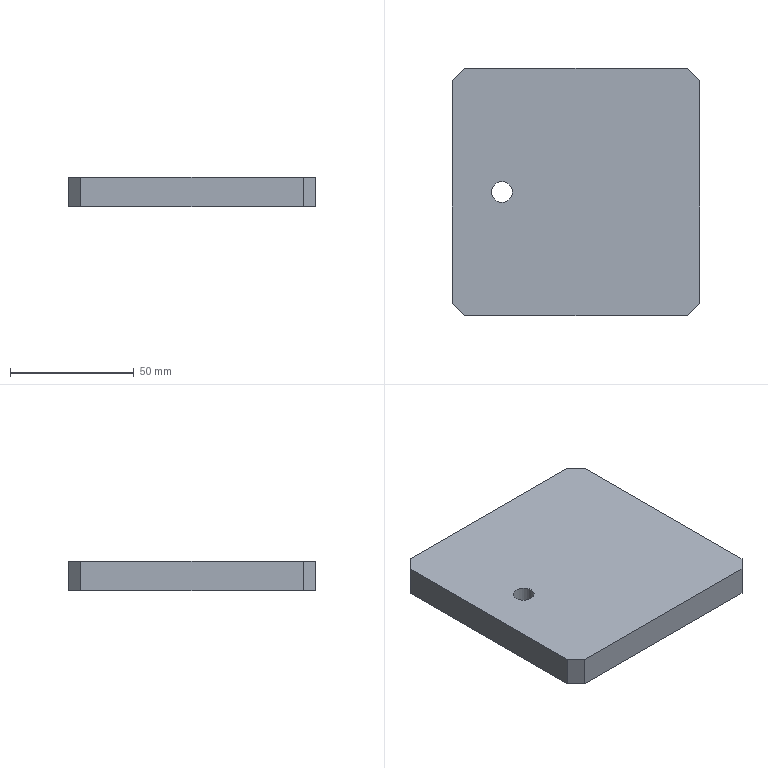Part | NX | features BREP 1 | 1 solid | 11 faces | box 100 x 100 x 12 mm | volume 118719 mm3 | plane 10 | cylinder 1 | commonest cylinder face diameters 8.5 x1
STEP:
#1=CARTESIAN_POINT('',(50.,-45.,12.));
#2=VERTEX_POINT('',#1);
#3=CARTESIAN_POINT('',(50.,45.,12.));
#4=VERTEX_POINT('',#3);
#5=CARTESIAN_POINT('',(50.,50.,12.));
#6=DIRECTION('',(0.,1.,0.));
#7=VECTOR('',#6,1000.);
#8=LINE('',#5,#7);
#9=EDGE_CURVE('',#2,#4,#8,.T.);
#10=ORIENTED_EDGE('',*,*,#9,.F.);
#11=CARTESIAN_POINT('',(50.,-45.,0.));
#12=VERTEX_POINT('',#11);
#13=CARTESIAN_POINT('',(50.,-45.,15.));
#14=DIRECTION('',(0.,0.,-1.));
#15=VECTOR('',#14,1000.);
#16=LINE('',#13,#15);
#17=EDGE_CURVE('',#2,#12,#16,.T.);
#18=ORIENTED_EDGE('',*,*,#17,.T.);
#19=CARTESIAN_POINT('',(50.,45.,0.));
#20=VERTEX_POINT('',#19);
#21=CARTESIAN_POINT('',(50.,50.,0.));
#22=DIRECTION('',(0.,1.,0.));
#23=VECTOR('',#22,1000.);
#24=LINE('',#21,#23);
#25=EDGE_CURVE('',#12,#20,#24,.T.);
#26=ORIENTED_EDGE('',*,*,#25,.T.);
#27=CARTESIAN_POINT('',(50.,45.,15.));
#28=DIRECTION('',(0.,0.,1.));
#29=VECTOR('',#28,1000.);
#30=LINE('',#27,#29);
#31=EDGE_CURVE('',#20,#4,#30,.T.);
#32=ORIENTED_EDGE('',*,*,#31,.T.);
#33=EDGE_LOOP('',(#10,#18,#26,#32));
#34=FACE_BOUND('',#33,.T.);
#35=CARTESIAN_POINT('',(50.,50.,15.));
#36=DIRECTION('',(-1.,0.,0.));
#37=DIRECTION('',(0.,0.,-1.));
#38=AXIS2_PLACEMENT_3D('',#35,#36,#37);
#39=PLANE('',#38);
#40=ADVANCED_FACE('',(#34),#39,.F.);
#41=CARTESIAN_POINT('',(45.,50.,12.));
#42=VERTEX_POINT('',#41);
#43=CARTESIAN_POINT('',(-45.,50.,12.));
#44=VERTEX_POINT('',#43);
#45=CARTESIAN_POINT('',(-50.,50.,12.));
#46=DIRECTION('',(-1.,0.,0.));
#47=VECTOR('',#46,1000.);
#48=LINE('',#45,#47);
#49=EDGE_CURVE('',#42,#44,#48,.T.);
#50=ORIENTED_EDGE('',*,*,#49,.F.);
#51=CARTESIAN_POINT('',(45.,50.,0.));
#52=VERTEX_POINT('',#51);
#53=CARTESIAN_POINT('',(45.,50.,15.));
#54=DIRECTION('',(0.,0.,-1.));
#55=VECTOR('',#54,1000.);
#56=LINE('',#53,#55);
#57=EDGE_CURVE('',#42,#52,#56,.T.);
#58=ORIENTED_EDGE('',*,*,#57,.T.);
#59=CARTESIAN_POINT('',(-45.,50.,0.));
#60=VERTEX_POINT('',#59);
#61=CARTESIAN_POINT('',(-50.,50.,0.));
#62=DIRECTION('',(-1.,0.,0.));
#63=VECTOR('',#62,1000.);
#64=LINE('',#61,#63);
#65=EDGE_CURVE('',#52,#60,#64,.T.);
#66=ORIENTED_EDGE('',*,*,#65,.T.);
#67=CARTESIAN_POINT('',(-45.,50.,15.));
#68=DIRECTION('',(0.,0.,1.));
#69=VECTOR('',#68,1000.);
#70=LINE('',#67,#69);
#71=EDGE_CURVE('',#60,#44,#70,.T.);
#72=ORIENTED_EDGE('',*,*,#71,.T.);
#73=EDGE_LOOP('',(#50,#58,#66,#72));
#74=FACE_BOUND('',#73,.T.);
#75=CARTESIAN_POINT('',(-50.,50.,15.));
#76=DIRECTION('',(0.,-1.,0.));
#77=DIRECTION('',(0.,0.,1.));
#78=AXIS2_PLACEMENT_3D('',#75,#76,#77);
#79=PLANE('',#78);
#80=ADVANCED_FACE('',(#74),#79,.F.);
#81=CARTESIAN_POINT('',(-50.,-45.,12.));
#82=VERTEX_POINT('',#81);
#83=CARTESIAN_POINT('',(-50.,45.,12.));
#84=VERTEX_POINT('',#83);
#85=CARTESIAN_POINT('',(-50.,-375.,12.));
#86=DIRECTION('',(0.,1.,0.));
#87=VECTOR('',#86,1000.);
#88=LINE('',#85,#87);
#89=EDGE_CURVE('',#82,#84,#88,.T.);
#90=ORIENTED_EDGE('',*,*,#89,.T.);
#91=CARTESIAN_POINT('',(-50.,45.,0.));
#92=VERTEX_POINT('',#91);
#93=CARTESIAN_POINT('',(-50.,45.,15.));
#94=DIRECTION('',(0.,0.,-1.));
#95=VECTOR('',#94,1000.);
#96=LINE('',#93,#95);
#97=EDGE_CURVE('',#84,#92,#96,.T.);
#98=ORIENTED_EDGE('',*,*,#97,.T.);
#99=CARTESIAN_POINT('',(-50.,-45.,0.));
#100=VERTEX_POINT('',#99);
#101=CARTESIAN_POINT('',(-50.,50.,0.));
#102=DIRECTION('',(0.,-1.,0.));
#103=VECTOR('',#102,1000.);
#104=LINE('',#101,#103);
#105=EDGE_CURVE('',#92,#100,#104,.T.);
#106=ORIENTED_EDGE('',*,*,#105,.T.);
#107=CARTESIAN_POINT('',(-50.,-45.,15.));
#108=DIRECTION('',(0.,0.,1.));
#109=VECTOR('',#108,1000.);
#110=LINE('',#107,#109);
#111=EDGE_CURVE('',#100,#82,#110,.T.);
#112=ORIENTED_EDGE('',*,*,#111,.T.);
#113=EDGE_LOOP('',(#90,#98,#106,#112));
#114=FACE_BOUND('',#113,.T.);
#115=CARTESIAN_POINT('',(-50.,50.,15.));
#116=DIRECTION('',(1.,0.,0.));
#117=DIRECTION('',(0.,-1.,0.));
#118=AXIS2_PLACEMENT_3D('',#115,#116,#117);
#119=PLANE('',#118);
#120=ADVANCED_FACE('',(#114),#119,.F.);
#121=CARTESIAN_POINT('',(-45.,-50.,12.));
#122=VERTEX_POINT('',#121);
#123=CARTESIAN_POINT('',(45.,-50.,12.));
#124=VERTEX_POINT('',#123);
#125=CARTESIAN_POINT('',(-50.,-50.,12.));
#126=DIRECTION('',(1.,0.,0.));
#127=VECTOR('',#126,1000.);
#128=LINE('',#125,#127);
#129=EDGE_CURVE('',#122,#124,#128,.T.);
#130=ORIENTED_EDGE('',*,*,#129,.F.);
#131=CARTESIAN_POINT('',(-45.,-50.,0.));
#132=VERTEX_POINT('',#131);
#133=CARTESIAN_POINT('',(-45.,-50.,15.));
#134=DIRECTION('',(0.,0.,-1.));
#135=VECTOR('',#134,1000.);
#136=LINE('',#133,#135);
#137=EDGE_CURVE('',#122,#132,#136,.T.);
#138=ORIENTED_EDGE('',*,*,#137,.T.);
#139=CARTESIAN_POINT('',(45.,-50.,0.));
#140=VERTEX_POINT('',#139);
#141=CARTESIAN_POINT('',(-50.,-50.,0.));
#142=DIRECTION('',(1.,0.,0.));
#143=VECTOR('',#142,1000.);
#144=LINE('',#141,#143);
#145=EDGE_CURVE('',#132,#140,#144,.T.);
#146=ORIENTED_EDGE('',*,*,#145,.T.);
#147=CARTESIAN_POINT('',(45.,-50.,15.));
#148=DIRECTION('',(0.,0.,1.));
#149=VECTOR('',#148,1000.);
#150=LINE('',#147,#149);
#151=EDGE_CURVE('',#140,#124,#150,.T.);
#152=ORIENTED_EDGE('',*,*,#151,.T.);
#153=EDGE_LOOP('',(#130,#138,#146,#152));
#154=FACE_BOUND('',#153,.T.);
#155=CARTESIAN_POINT('',(-50.,-50.,15.));
#156=DIRECTION('',(0.,1.,0.));
#157=DIRECTION('',(0.,0.,-1.));
#158=AXIS2_PLACEMENT_3D('',#155,#156,#157);
#159=PLANE('',#158);
#160=ADVANCED_FACE('',(#154),#159,.F.);
#161=ORIENTED_EDGE('',*,*,#137,.F.);
#162=CARTESIAN_POINT('',(-45.,-50.,12.));
#163=DIRECTION('',(-0.7071,0.7071,0.));
#164=VECTOR('',#163,1000.);
#165=LINE('',#162,#164);
#166=EDGE_CURVE('',#122,#82,#165,.T.);
#167=ORIENTED_EDGE('',*,*,#166,.T.);
#168=ORIENTED_EDGE('',*,*,#111,.F.);
#169=CARTESIAN_POINT('',(-45.,-50.,0.));
#170=DIRECTION('',(-0.7071,0.7071,0.));
#171=VECTOR('',#170,1000.);
#172=LINE('',#169,#171);
#173=EDGE_CURVE('',#132,#100,#172,.T.);
#174=ORIENTED_EDGE('',*,*,#173,.F.);
#175=EDGE_LOOP('',(#161,#167,#168,#174));
#176=FACE_BOUND('',#175,.T.);
#177=CARTESIAN_POINT('',(-45.,-50.,15.));
#178=DIRECTION('',(0.7071,0.7071,0.));
#179=DIRECTION('',(0.,0.,1.));
#180=AXIS2_PLACEMENT_3D('',#177,#178,#179);
#181=PLANE('',#180);
#182=ADVANCED_FACE('',(#176),#181,.F.);
#183=ORIENTED_EDGE('',*,*,#17,.F.);
#184=CARTESIAN_POINT('',(50.,-45.,12.));
#185=DIRECTION('',(-0.7071,-0.7071,0.));
#186=VECTOR('',#185,1000.);
#187=LINE('',#184,#186);
#188=EDGE_CURVE('',#2,#124,#187,.T.);
#189=ORIENTED_EDGE('',*,*,#188,.T.);
#190=ORIENTED_EDGE('',*,*,#151,.F.);
#191=CARTESIAN_POINT('',(50.,-45.,0.));
#192=DIRECTION('',(-0.7071,-0.7071,0.));
#193=VECTOR('',#192,1000.);
#194=LINE('',#191,#193);
#195=EDGE_CURVE('',#12,#140,#194,.T.);
#196=ORIENTED_EDGE('',*,*,#195,.F.);
#197=EDGE_LOOP('',(#183,#189,#190,#196));
#198=FACE_BOUND('',#197,.T.);
#199=CARTESIAN_POINT('',(50.,-45.,15.));
#200=DIRECTION('',(-0.7071,0.7071,0.));
#201=DIRECTION('',(0.,0.,1.));
#202=AXIS2_PLACEMENT_3D('',#199,#200,#201);
#203=PLANE('',#202);
#204=ADVANCED_FACE('',(#198),#203,.F.);
#205=ORIENTED_EDGE('',*,*,#57,.F.);
#206=CARTESIAN_POINT('',(45.,50.,12.));
#207=DIRECTION('',(0.7071,-0.7071,0.));
#208=VECTOR('',#207,1000.);
#209=LINE('',#206,#208);
#210=EDGE_CURVE('',#42,#4,#209,.T.);
#211=ORIENTED_EDGE('',*,*,#210,.T.);
#212=ORIENTED_EDGE('',*,*,#31,.F.);
#213=CARTESIAN_POINT('',(45.,50.,0.));
#214=DIRECTION('',(0.7071,-0.7071,0.));
#215=VECTOR('',#214,1000.);
#216=LINE('',#213,#215);
#217=EDGE_CURVE('',#52,#20,#216,.T.);
#218=ORIENTED_EDGE('',*,*,#217,.F.);
#219=EDGE_LOOP('',(#205,#211,#212,#218));
#220=FACE_BOUND('',#219,.T.);
#221=CARTESIAN_POINT('',(45.,50.,15.));
#222=DIRECTION('',(-0.7071,-0.7071,0.));
#223=DIRECTION('',(0.,0.,1.));
#224=AXIS2_PLACEMENT_3D('',#221,#222,#223);
#225=PLANE('',#224);
#226=ADVANCED_FACE('',(#220),#225,.F.);
#227=ORIENTED_EDGE('',*,*,#97,.F.);
#228=CARTESIAN_POINT('',(-50.,45.,12.));
#229=DIRECTION('',(0.7071,0.7071,0.));
#230=VECTOR('',#229,1000.);
#231=LINE('',#228,#230);
#232=EDGE_CURVE('',#84,#44,#231,.T.);
#233=ORIENTED_EDGE('',*,*,#232,.T.);
#234=ORIENTED_EDGE('',*,*,#71,.F.);
#235=CARTESIAN_POINT('',(-50.,45.,0.));
#236=DIRECTION('',(0.7071,0.7071,0.));
#237=VECTOR('',#236,1000.);
#238=LINE('',#235,#237);
#239=EDGE_CURVE('',#92,#60,#238,.T.);
#240=ORIENTED_EDGE('',*,*,#239,.F.);
#241=EDGE_LOOP('',(#227,#233,#234,#240));
#242=FACE_BOUND('',#241,.T.);
#243=CARTESIAN_POINT('',(-50.,45.,15.));
#244=DIRECTION('',(0.7071,-0.7071,0.));
#245=DIRECTION('',(0.,0.,1.));
#246=AXIS2_PLACEMENT_3D('',#243,#244,#245);
#247=PLANE('',#246);
#248=ADVANCED_FACE('',(#242),#247,.F.);
#249=CARTESIAN_POINT('',(-25.75,0.,0.));
#250=VERTEX_POINT('',#249);
#251=CARTESIAN_POINT('',(-30.,0.,0.));
#252=DIRECTION('',(0.,0.,1.));
#253=DIRECTION('',(1.,0.,0.));
#254=AXIS2_PLACEMENT_3D('',#251,#252,#253);
#255=CIRCLE('',#254,4.25);
#256=EDGE_CURVE('',#250,#250,#255,.T.);
#257=ORIENTED_EDGE('',*,*,#256,.T.);
#258=EDGE_LOOP('',(#257));
#259=FACE_BOUND('',#258,.T.);
#260=ORIENTED_EDGE('',*,*,#145,.F.);
#261=ORIENTED_EDGE('',*,*,#173,.T.);
#262=ORIENTED_EDGE('',*,*,#105,.F.);
#263=ORIENTED_EDGE('',*,*,#239,.T.);
#264=ORIENTED_EDGE('',*,*,#65,.F.);
#265=ORIENTED_EDGE('',*,*,#217,.T.);
#266=ORIENTED_EDGE('',*,*,#25,.F.);
#267=ORIENTED_EDGE('',*,*,#195,.T.);
#268=EDGE_LOOP('',(#260,#261,#262,#263,#264,#265,#266,#267));
#269=FACE_BOUND('',#268,.T.);
#270=CARTESIAN_POINT('',(0.,0.,0.));
#271=DIRECTION('',(0.,0.,1.));
#272=DIRECTION('',(-1.,0.,0.));
#273=AXIS2_PLACEMENT_3D('',#270,#271,#272);
#274=PLANE('',#273);
#275=ADVANCED_FACE('',(#259,#269),#274,.F.);
#276=CARTESIAN_POINT('',(-25.75,0.,12.));
#277=VERTEX_POINT('',#276);
#278=CARTESIAN_POINT('',(-30.,0.,12.));
#279=DIRECTION('',(0.,0.,1.));
#280=DIRECTION('',(1.,0.,0.));
#281=AXIS2_PLACEMENT_3D('',#278,#279,#280);
#282=CIRCLE('',#281,4.25);
#283=EDGE_CURVE('',#277,#277,#282,.T.);
#284=ORIENTED_EDGE('',*,*,#283,.F.);
#285=EDGE_LOOP('',(#284));
#286=FACE_BOUND('',#285,.T.);
#287=ORIENTED_EDGE('',*,*,#129,.T.);
#288=ORIENTED_EDGE('',*,*,#188,.F.);
#289=ORIENTED_EDGE('',*,*,#9,.T.);
#290=ORIENTED_EDGE('',*,*,#210,.F.);
#291=ORIENTED_EDGE('',*,*,#49,.T.);
#292=ORIENTED_EDGE('',*,*,#232,.F.);
#293=ORIENTED_EDGE('',*,*,#89,.F.);
#294=ORIENTED_EDGE('',*,*,#166,.F.);
#295=EDGE_LOOP('',(#287,#288,#289,#290,#291,#292,#293,#294));
#296=FACE_BOUND('',#295,.T.);
#297=CARTESIAN_POINT('',(900.,-25.,12.));
#298=DIRECTION('',(0.,0.,1.));
#299=DIRECTION('',(-1.,0.,0.));
#300=AXIS2_PLACEMENT_3D('',#297,#298,#299);
#301=PLANE('',#300);
#302=ADVANCED_FACE('',(#286,#296),#301,.T.);
#303=ORIENTED_EDGE('',*,*,#283,.T.);
#304=EDGE_LOOP('',(#303));
#305=FACE_BOUND('',#304,.T.);
#306=ORIENTED_EDGE('',*,*,#256,.F.);
#307=EDGE_LOOP('',(#306));
#308=FACE_BOUND('',#307,.T.);
#309=CARTESIAN_POINT('',(-30.,0.,12.));
#310=DIRECTION('',(0.,0.,1.));
#311=DIRECTION('',(-1.,0.,0.));
#312=AXIS2_PLACEMENT_3D('',#309,#310,#311);
#313=CYLINDRICAL_SURFACE('',#312,4.25);
#314=ADVANCED_FACE('',(#305,#308),#313,.F.);
#315=CLOSED_SHELL('',(#40,#80,#120,#160,#182,#204,#226,#248,#275,#302,#314));
#316=MANIFOLD_SOLID_BREP('',#315);
#317=(LENGTH_UNIT()NAMED_UNIT(*)SI_UNIT(.MILLI.,.METRE.));
#318=UNCERTAINTY_MEASURE_WITH_UNIT(LENGTH_MEASURE(0.00001),#317,'','');
#319=(NAMED_UNIT(*)PLANE_ANGLE_UNIT()SI_UNIT($,.RADIAN.));
#320=(NAMED_UNIT(*)SI_UNIT($,.STERADIAN.)SOLID_ANGLE_UNIT());
#321=(GEOMETRIC_REPRESENTATION_CONTEXT(3)GLOBAL_UNCERTAINTY_ASSIGNED_CONTEXT((#318))GLOBAL_UNIT_ASSIGNED_CONTEXT((#317,#319,#320))REPRESENTATION_CONTEXT('',''));
#322=ADVANCED_BREP_SHAPE_REPRESENTATION('',(#316),#321);